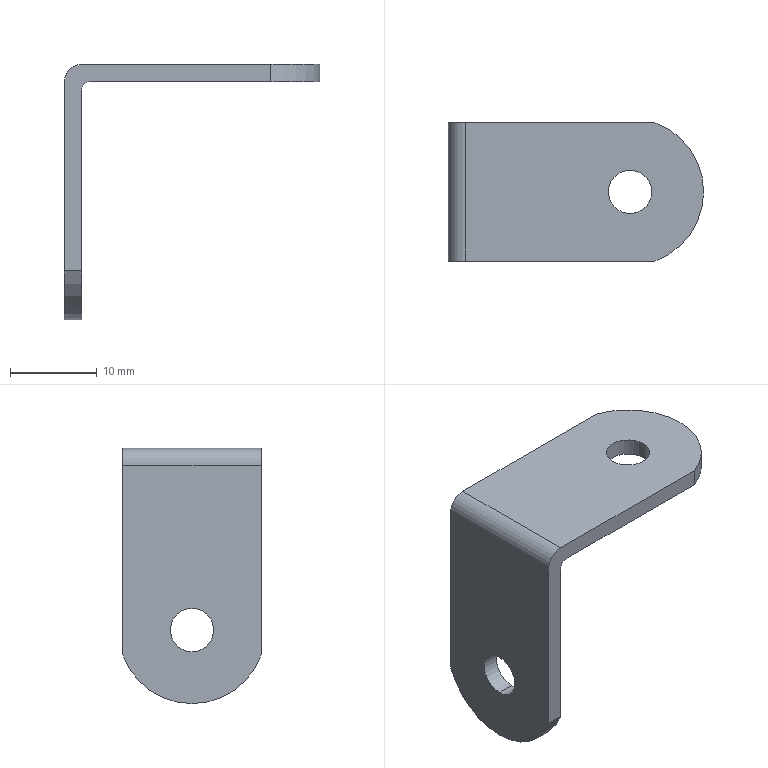Part | SolidWorks | features BaseBody 1 | 1 solid | 15 faces | box 29.5 x 16 x 29.5 mm | volume 1637 mm3 | cylinder 9 | plane 6 | commonest cylinder face diameters 5 x4 17 x3 2 x1 4 x1
STEP:
#1=CARTESIAN_POINT('',(-1.,-8.,-22.872));
#2=VERTEX_POINT('',#1);
#3=CARTESIAN_POINT('',(-1.,0.,-28.5));
#4=VERTEX_POINT('',#3);
#5=CARTESIAN_POINT('',(-1.,0.,-20.));
#6=DIRECTION('',(1.,0.,0.));
#7=DIRECTION('',(0.,0.,-1.));
#8=AXIS2_PLACEMENT_3D('',#5,#6,#7);
#9=CIRCLE('',#8,8.5);
#10=EDGE_CURVE('',#2,#4,#9,.T.);
#11=ORIENTED_EDGE('',*,*,#10,.T.);
#12=CARTESIAN_POINT('',(1.,0.,-28.5));
#13=VERTEX_POINT('',#12);
#14=CARTESIAN_POINT('',(-15.,0.,-28.5));
#15=DIRECTION('',(1.,0.,0.));
#16=VECTOR('',#15,1000.);
#17=LINE('',#14,#16);
#18=EDGE_CURVE('',#4,#13,#17,.T.);
#19=ORIENTED_EDGE('',*,*,#18,.T.);
#20=CARTESIAN_POINT('',(1.,-8.,-22.872));
#21=VERTEX_POINT('',#20);
#22=CARTESIAN_POINT('',(1.,0.,-20.));
#23=DIRECTION('',(-1.,0.,0.));
#24=DIRECTION('',(0.,0.,-1.));
#25=AXIS2_PLACEMENT_3D('',#22,#23,#24);
#26=CIRCLE('',#25,8.5);
#27=EDGE_CURVE('',#13,#21,#26,.T.);
#28=ORIENTED_EDGE('',*,*,#27,.T.);
#29=CARTESIAN_POINT('',(0.,-8.,-22.872));
#30=DIRECTION('',(1.,0.,0.));
#31=VECTOR('',#30,1000.);
#32=LINE('',#29,#31);
#33=EDGE_CURVE('',#2,#21,#32,.T.);
#34=ORIENTED_EDGE('',*,*,#33,.F.);
#35=EDGE_LOOP('',(#11,#19,#28,#34));
#36=FACE_OUTER_BOUND('',#35,.T.);
#37=CARTESIAN_POINT('',(-15.,0.,-20.));
#38=DIRECTION('',(1.,0.,0.));
#39=DIRECTION('',(0.,0.,-1.));
#40=AXIS2_PLACEMENT_3D('',#37,#38,#39);
#41=CYLINDRICAL_SURFACE('',#40,8.5);
#42=ADVANCED_FACE('',(#36),#41,.T.);
#43=CARTESIAN_POINT('',(-1.,0.,-22.5));
#44=VERTEX_POINT('',#43);
#45=CARTESIAN_POINT('',(-1.,0.,-17.5));
#46=VERTEX_POINT('',#45);
#47=CARTESIAN_POINT('',(-1.,0.,-20.));
#48=DIRECTION('',(-1.,0.,0.));
#49=DIRECTION('',(0.,0.,-1.));
#50=AXIS2_PLACEMENT_3D('',#47,#48,#49);
#51=CIRCLE('',#50,2.5);
#52=EDGE_CURVE('',#44,#46,#51,.T.);
#53=ORIENTED_EDGE('',*,*,#52,.T.);
#54=CARTESIAN_POINT('',(1.,0.,-17.5));
#55=VERTEX_POINT('',#54);
#56=CARTESIAN_POINT('',(-15.,0.,-17.5));
#57=DIRECTION('',(1.,0.,0.));
#58=VECTOR('',#57,1000.);
#59=LINE('',#56,#58);
#60=EDGE_CURVE('',#46,#55,#59,.T.);
#61=ORIENTED_EDGE('',*,*,#60,.T.);
#62=CARTESIAN_POINT('',(1.,0.,-22.5));
#63=VERTEX_POINT('',#62);
#64=CARTESIAN_POINT('',(1.,0.,-20.));
#65=DIRECTION('',(-1.,0.,0.));
#66=DIRECTION('',(0.,0.,-1.));
#67=AXIS2_PLACEMENT_3D('',#64,#65,#66);
#68=CIRCLE('',#67,2.5);
#69=EDGE_CURVE('',#63,#55,#68,.T.);
#70=ORIENTED_EDGE('',*,*,#69,.F.);
#71=CARTESIAN_POINT('',(-15.,0.,-22.5));
#72=DIRECTION('',(1.,0.,0.));
#73=VECTOR('',#72,1000.);
#74=LINE('',#71,#73);
#75=EDGE_CURVE('',#44,#63,#74,.T.);
#76=ORIENTED_EDGE('',*,*,#75,.F.);
#77=EDGE_LOOP('',(#53,#61,#70,#76));
#78=FACE_OUTER_BOUND('',#77,.T.);
#79=CARTESIAN_POINT('',(-15.,0.,-20.));
#80=DIRECTION('',(1.,0.,0.));
#81=DIRECTION('',(0.,0.,-1.));
#82=AXIS2_PLACEMENT_3D('',#79,#80,#81);
#83=CYLINDRICAL_SURFACE('',#82,2.5);
#84=ADVANCED_FACE('',(#78),#83,.F.);
#85=CARTESIAN_POINT('',(17.5,0.,1.));
#86=VERTEX_POINT('',#85);
#87=CARTESIAN_POINT('',(22.5,0.,1.));
#88=VERTEX_POINT('',#87);
#89=CARTESIAN_POINT('',(20.,0.,1.));
#90=DIRECTION('',(0.,0.,1.));
#91=DIRECTION('',(-1.,0.,0.));
#92=AXIS2_PLACEMENT_3D('',#89,#90,#91);
#93=CIRCLE('',#92,2.5);
#94=EDGE_CURVE('',#86,#88,#93,.T.);
#95=ORIENTED_EDGE('',*,*,#94,.T.);
#96=CARTESIAN_POINT('',(22.5,0.,-1.));
#97=VERTEX_POINT('',#96);
#98=CARTESIAN_POINT('',(22.5,0.,15.));
#99=DIRECTION('',(0.,0.,-1.));
#100=VECTOR('',#99,1000.);
#101=LINE('',#98,#100);
#102=EDGE_CURVE('',#88,#97,#101,.T.);
#103=ORIENTED_EDGE('',*,*,#102,.T.);
#104=CARTESIAN_POINT('',(17.5,0.,-1.));
#105=VERTEX_POINT('',#104);
#106=CARTESIAN_POINT('',(20.,0.,-1.));
#107=DIRECTION('',(0.,0.,-1.));
#108=DIRECTION('',(-1.,0.,0.));
#109=AXIS2_PLACEMENT_3D('',#106,#107,#108);
#110=CIRCLE('',#109,2.5);
#111=EDGE_CURVE('',#97,#105,#110,.T.);
#112=ORIENTED_EDGE('',*,*,#111,.T.);
#113=CARTESIAN_POINT('',(17.5,0.,15.));
#114=DIRECTION('',(0.,0.,-1.));
#115=VECTOR('',#114,1000.);
#116=LINE('',#113,#115);
#117=EDGE_CURVE('',#86,#105,#116,.T.);
#118=ORIENTED_EDGE('',*,*,#117,.F.);
#119=EDGE_LOOP('',(#95,#103,#112,#118));
#120=FACE_OUTER_BOUND('',#119,.T.);
#121=CARTESIAN_POINT('',(20.,0.,15.));
#122=DIRECTION('',(0.,0.,-1.));
#123=DIRECTION('',(-1.,0.,0.));
#124=AXIS2_PLACEMENT_3D('',#121,#122,#123);
#125=CYLINDRICAL_SURFACE('',#124,2.5);
#126=ADVANCED_FACE('',(#120),#125,.F.);
#127=CARTESIAN_POINT('',(-1.,8.,-1.));
#128=VERTEX_POINT('',#127);
#129=CARTESIAN_POINT('',(-1.,-8.,-1.));
#130=VERTEX_POINT('',#129);
#131=CARTESIAN_POINT('',(-1.,8.,-1.));
#132=DIRECTION('',(0.,-1.,0.));
#133=VECTOR('',#132,1000.);
#134=LINE('',#131,#133);
#135=EDGE_CURVE('',#128,#130,#134,.T.);
#136=ORIENTED_EDGE('',*,*,#135,.F.);
#137=CARTESIAN_POINT('',(-1.,8.,-22.872));
#138=VERTEX_POINT('',#137);
#139=CARTESIAN_POINT('',(-1.,8.,1.));
#140=DIRECTION('',(0.,0.,1.));
#141=VECTOR('',#140,1000.);
#142=LINE('',#139,#141);
#143=EDGE_CURVE('',#138,#128,#142,.T.);
#144=ORIENTED_EDGE('',*,*,#143,.F.);
#145=CARTESIAN_POINT('',(-1.,0.,-20.));
#146=DIRECTION('',(1.,0.,0.));
#147=DIRECTION('',(0.,0.,-1.));
#148=AXIS2_PLACEMENT_3D('',#145,#146,#147);
#149=CIRCLE('',#148,8.5);
#150=EDGE_CURVE('',#4,#138,#149,.T.);
#151=ORIENTED_EDGE('',*,*,#150,.F.);
#152=ORIENTED_EDGE('',*,*,#10,.F.);
#153=CARTESIAN_POINT('',(-1.,-8.,1.));
#154=DIRECTION('',(0.,0.,-1.));
#155=VECTOR('',#154,1000.);
#156=LINE('',#153,#155);
#157=EDGE_CURVE('',#130,#2,#156,.T.);
#158=ORIENTED_EDGE('',*,*,#157,.F.);
#159=EDGE_LOOP('',(#136,#144,#151,#152,#158));
#160=FACE_OUTER_BOUND('',#159,.T.);
#161=ORIENTED_EDGE('',*,*,#52,.F.);
#162=CARTESIAN_POINT('',(-1.,0.,-20.));
#163=DIRECTION('',(-1.,0.,0.));
#164=DIRECTION('',(0.,0.,-1.));
#165=AXIS2_PLACEMENT_3D('',#162,#163,#164);
#166=CIRCLE('',#165,2.5);
#167=EDGE_CURVE('',#46,#44,#166,.T.);
#168=ORIENTED_EDGE('',*,*,#167,.F.);
#169=EDGE_LOOP('',(#161,#168));
#170=FACE_BOUND('',#169,.T.);
#171=CARTESIAN_POINT('',(-1.,8.,1.));
#172=DIRECTION('',(1.,0.,0.));
#173=DIRECTION('',(0.,0.,-1.));
#174=AXIS2_PLACEMENT_3D('',#171,#172,#173);
#175=PLANE('',#174);
#176=ADVANCED_FACE('',(#160,#170),#175,.F.);
#177=CARTESIAN_POINT('',(2.,-8.,-1.));
#178=VERTEX_POINT('',#177);
#179=CARTESIAN_POINT('',(22.872,-8.,-1.));
#180=VERTEX_POINT('',#179);
#181=CARTESIAN_POINT('',(0.,-8.,-1.));
#182=DIRECTION('',(1.,0.,0.));
#183=VECTOR('',#182,1000.);
#184=LINE('',#181,#183);
#185=EDGE_CURVE('',#178,#180,#184,.T.);
#186=ORIENTED_EDGE('',*,*,#185,.T.);
#187=CARTESIAN_POINT('',(22.872,-8.,1.));
#188=VERTEX_POINT('',#187);
#189=CARTESIAN_POINT('',(22.872,-8.,0.));
#190=DIRECTION('',(0.,0.,1.));
#191=VECTOR('',#190,1000.);
#192=LINE('',#189,#191);
#193=EDGE_CURVE('',#180,#188,#192,.T.);
#194=ORIENTED_EDGE('',*,*,#193,.T.);
#195=CARTESIAN_POINT('',(1.,-8.,1.));
#196=VERTEX_POINT('',#195);
#197=CARTESIAN_POINT('',(0.,-8.,1.));
#198=DIRECTION('',(-1.,0.,0.));
#199=VECTOR('',#198,1000.);
#200=LINE('',#197,#199);
#201=EDGE_CURVE('',#188,#196,#200,.T.);
#202=ORIENTED_EDGE('',*,*,#201,.T.);
#203=CARTESIAN_POINT('',(1.,-8.,-1.));
#204=DIRECTION('',(0.,-1.,0.));
#205=DIRECTION('',(0.,0.,-1.));
#206=AXIS2_PLACEMENT_3D('',#203,#204,#205);
#207=CIRCLE('',#206,2.);
#208=EDGE_CURVE('',#196,#130,#207,.T.);
#209=ORIENTED_EDGE('',*,*,#208,.T.);
#210=ORIENTED_EDGE('',*,*,#157,.T.);
#211=ORIENTED_EDGE('',*,*,#33,.T.);
#212=CARTESIAN_POINT('',(1.,-8.,-2.));
#213=VERTEX_POINT('',#212);
#214=CARTESIAN_POINT('',(1.,-8.,0.));
#215=DIRECTION('',(0.,0.,1.));
#216=VECTOR('',#215,1000.);
#217=LINE('',#214,#216);
#218=EDGE_CURVE('',#21,#213,#217,.T.);
#219=ORIENTED_EDGE('',*,*,#218,.T.);
#220=CARTESIAN_POINT('',(2.,-8.,-2.));
#221=DIRECTION('',(0.,1.,0.));
#222=DIRECTION('',(0.,0.,1.));
#223=AXIS2_PLACEMENT_3D('',#220,#221,#222);
#224=CIRCLE('',#223,1.);
#225=EDGE_CURVE('',#213,#178,#224,.T.);
#226=ORIENTED_EDGE('',*,*,#225,.T.);
#227=EDGE_LOOP('',(#186,#194,#202,#209,#210,#211,#219,#226));
#228=FACE_OUTER_BOUND('',#227,.T.);
#229=CARTESIAN_POINT('',(0.,-8.,0.));
#230=DIRECTION('',(0.,-1.,0.));
#231=DIRECTION('',(0.,0.,-1.));
#232=AXIS2_PLACEMENT_3D('',#229,#230,#231);
#233=PLANE('',#232);
#234=ADVANCED_FACE('',(#228),#233,.T.);
#235=ORIENTED_EDGE('',*,*,#208,.F.);
#236=CARTESIAN_POINT('',(1.,8.,1.));
#237=VERTEX_POINT('',#236);
#238=CARTESIAN_POINT('',(1.,8.,1.));
#239=DIRECTION('',(0.,1.,0.));
#240=VECTOR('',#239,1000.);
#241=LINE('',#238,#240);
#242=EDGE_CURVE('',#196,#237,#241,.T.);
#243=ORIENTED_EDGE('',*,*,#242,.T.);
#244=CARTESIAN_POINT('',(1.,8.,-1.));
#245=DIRECTION('',(0.,-1.,0.));
#246=DIRECTION('',(0.,0.,-1.));
#247=AXIS2_PLACEMENT_3D('',#244,#245,#246);
#248=CIRCLE('',#247,2.);
#249=EDGE_CURVE('',#237,#128,#248,.T.);
#250=ORIENTED_EDGE('',*,*,#249,.T.);
#251=ORIENTED_EDGE('',*,*,#135,.T.);
#252=EDGE_LOOP('',(#235,#243,#250,#251));
#253=FACE_OUTER_BOUND('',#252,.T.);
#254=CARTESIAN_POINT('',(1.,8.,-1.));
#255=DIRECTION('',(0.,-1.,0.));
#256=DIRECTION('',(0.,0.,-1.));
#257=AXIS2_PLACEMENT_3D('',#254,#255,#256);
#258=CYLINDRICAL_SURFACE('',#257,2.);
#259=ADVANCED_FACE('',(#253),#258,.T.);
#260=ORIENTED_EDGE('',*,*,#249,.F.);
#261=CARTESIAN_POINT('',(22.872,8.,1.));
#262=VERTEX_POINT('',#261);
#263=CARTESIAN_POINT('',(0.,8.,1.));
#264=DIRECTION('',(-1.,0.,0.));
#265=VECTOR('',#264,1000.);
#266=LINE('',#263,#265);
#267=EDGE_CURVE('',#262,#237,#266,.T.);
#268=ORIENTED_EDGE('',*,*,#267,.F.);
#269=CARTESIAN_POINT('',(22.872,8.,-1.));
#270=VERTEX_POINT('',#269);
#271=CARTESIAN_POINT('',(22.872,8.,0.));
#272=DIRECTION('',(0.,0.,1.));
#273=VECTOR('',#272,1000.);
#274=LINE('',#271,#273);
#275=EDGE_CURVE('',#270,#262,#274,.T.);
#276=ORIENTED_EDGE('',*,*,#275,.F.);
#277=CARTESIAN_POINT('',(2.,8.,-1.));
#278=VERTEX_POINT('',#277);
#279=CARTESIAN_POINT('',(0.,8.,-1.));
#280=DIRECTION('',(1.,0.,0.));
#281=VECTOR('',#280,1000.);
#282=LINE('',#279,#281);
#283=EDGE_CURVE('',#278,#270,#282,.T.);
#284=ORIENTED_EDGE('',*,*,#283,.F.);
#285=CARTESIAN_POINT('',(1.,8.,-2.));
#286=VERTEX_POINT('',#285);
#287=CARTESIAN_POINT('',(2.,8.,-2.));
#288=DIRECTION('',(0.,-1.,0.));
#289=DIRECTION('',(0.,0.,1.));
#290=AXIS2_PLACEMENT_3D('',#287,#288,#289);
#291=CIRCLE('',#290,1.);
#292=EDGE_CURVE('',#278,#286,#291,.T.);
#293=ORIENTED_EDGE('',*,*,#292,.T.);
#294=CARTESIAN_POINT('',(1.,8.,-22.872));
#295=VERTEX_POINT('',#294);
#296=CARTESIAN_POINT('',(1.,8.,0.));
#297=DIRECTION('',(0.,0.,1.));
#298=VECTOR('',#297,1000.);
#299=LINE('',#296,#298);
#300=EDGE_CURVE('',#295,#286,#299,.T.);
#301=ORIENTED_EDGE('',*,*,#300,.F.);
#302=CARTESIAN_POINT('',(0.,8.,-22.872));
#303=DIRECTION('',(1.,0.,0.));
#304=VECTOR('',#303,1000.);
#305=LINE('',#302,#304);
#306=EDGE_CURVE('',#138,#295,#305,.T.);
#307=ORIENTED_EDGE('',*,*,#306,.F.);
#308=ORIENTED_EDGE('',*,*,#143,.T.);
#309=EDGE_LOOP('',(#260,#268,#276,#284,#293,#301,#307,#308));
#310=FACE_OUTER_BOUND('',#309,.T.);
#311=CARTESIAN_POINT('',(0.,8.,0.));
#312=DIRECTION('',(0.,-1.,0.));
#313=DIRECTION('',(0.,0.,-1.));
#314=AXIS2_PLACEMENT_3D('',#311,#312,#313);
#315=PLANE('',#314);
#316=ADVANCED_FACE('',(#310),#315,.F.);
#317=ORIENTED_EDGE('',*,*,#18,.F.);
#318=ORIENTED_EDGE('',*,*,#150,.T.);
#319=ORIENTED_EDGE('',*,*,#306,.T.);
#320=CARTESIAN_POINT('',(1.,0.,-20.));
#321=DIRECTION('',(-1.,0.,0.));
#322=DIRECTION('',(0.,0.,-1.));
#323=AXIS2_PLACEMENT_3D('',#320,#321,#322);
#324=CIRCLE('',#323,8.5);
#325=EDGE_CURVE('',#295,#13,#324,.T.);
#326=ORIENTED_EDGE('',*,*,#325,.T.);
#327=EDGE_LOOP('',(#317,#318,#319,#326));
#328=FACE_OUTER_BOUND('',#327,.T.);
#329=CARTESIAN_POINT('',(-15.,0.,-20.));
#330=DIRECTION('',(1.,0.,0.));
#331=DIRECTION('',(0.,0.,-1.));
#332=AXIS2_PLACEMENT_3D('',#329,#330,#331);
#333=CYLINDRICAL_SURFACE('',#332,8.5);
#334=ADVANCED_FACE('',(#328),#333,.T.);
#335=ORIENTED_EDGE('',*,*,#60,.F.);
#336=ORIENTED_EDGE('',*,*,#167,.T.);
#337=ORIENTED_EDGE('',*,*,#75,.T.);
#338=CARTESIAN_POINT('',(1.,0.,-20.));
#339=DIRECTION('',(-1.,0.,0.));
#340=DIRECTION('',(0.,0.,-1.));
#341=AXIS2_PLACEMENT_3D('',#338,#339,#340);
#342=CIRCLE('',#341,2.5);
#343=EDGE_CURVE('',#55,#63,#342,.T.);
#344=ORIENTED_EDGE('',*,*,#343,.F.);
#345=EDGE_LOOP('',(#335,#336,#337,#344));
#346=FACE_OUTER_BOUND('',#345,.T.);
#347=CARTESIAN_POINT('',(-15.,0.,-20.));
#348=DIRECTION('',(1.,0.,0.));
#349=DIRECTION('',(0.,0.,-1.));
#350=AXIS2_PLACEMENT_3D('',#347,#348,#349);
#351=CYLINDRICAL_SURFACE('',#350,2.5);
#352=ADVANCED_FACE('',(#346),#351,.F.);
#353=ORIENTED_EDGE('',*,*,#275,.T.);
#354=CARTESIAN_POINT('',(20.,0.,1.));
#355=DIRECTION('',(0.,0.,-1.));
#356=DIRECTION('',(-1.,0.,0.));
#357=AXIS2_PLACEMENT_3D('',#354,#355,#356);
#358=CIRCLE('',#357,8.5);
#359=EDGE_CURVE('',#262,#188,#358,.T.);
#360=ORIENTED_EDGE('',*,*,#359,.T.);
#361=ORIENTED_EDGE('',*,*,#193,.F.);
#362=CARTESIAN_POINT('',(20.,0.,-1.));
#363=DIRECTION('',(0.,0.,1.));
#364=DIRECTION('',(-1.,0.,0.));
#365=AXIS2_PLACEMENT_3D('',#362,#363,#364);
#366=CIRCLE('',#365,8.5);
#367=EDGE_CURVE('',#180,#270,#366,.T.);
#368=ORIENTED_EDGE('',*,*,#367,.T.);
#369=EDGE_LOOP('',(#353,#360,#361,#368));
#370=FACE_OUTER_BOUND('',#369,.T.);
#371=CARTESIAN_POINT('',(20.,0.,15.));
#372=DIRECTION('',(0.,0.,-1.));
#373=DIRECTION('',(-1.,0.,0.));
#374=AXIS2_PLACEMENT_3D('',#371,#372,#373);
#375=CYLINDRICAL_SURFACE('',#374,8.5);
#376=ADVANCED_FACE('',(#370),#375,.T.);
#377=CARTESIAN_POINT('',(2.,8.,-1.));
#378=DIRECTION('',(0.,-1.,0.));
#379=VECTOR('',#378,1000.);
#380=LINE('',#377,#379);
#381=EDGE_CURVE('',#278,#178,#380,.T.);
#382=ORIENTED_EDGE('',*,*,#381,.F.);
#383=ORIENTED_EDGE('',*,*,#283,.T.);
#384=ORIENTED_EDGE('',*,*,#367,.F.);
#385=ORIENTED_EDGE('',*,*,#185,.F.);
#386=EDGE_LOOP('',(#382,#383,#384,#385));
#387=FACE_OUTER_BOUND('',#386,.T.);
#388=CARTESIAN_POINT('',(20.,0.,-1.));
#389=DIRECTION('',(0.,0.,-1.));
#390=DIRECTION('',(-1.,0.,0.));
#391=AXIS2_PLACEMENT_3D('',#388,#389,#390);
#392=CIRCLE('',#391,2.5);
#393=EDGE_CURVE('',#105,#97,#392,.T.);
#394=ORIENTED_EDGE('',*,*,#393,.F.);
#395=ORIENTED_EDGE('',*,*,#111,.F.);
#396=EDGE_LOOP('',(#394,#395));
#397=FACE_BOUND('',#396,.T.);
#398=CARTESIAN_POINT('',(1.,8.,-1.));
#399=DIRECTION('',(0.,0.,1.));
#400=DIRECTION('',(1.,0.,0.));
#401=AXIS2_PLACEMENT_3D('',#398,#399,#400);
#402=PLANE('',#401);
#403=ADVANCED_FACE('',(#387,#397),#402,.F.);
#404=CARTESIAN_POINT('',(1.,8.,-2.));
#405=DIRECTION('',(0.,1.,0.));
#406=VECTOR('',#405,1000.);
#407=LINE('',#404,#406);
#408=EDGE_CURVE('',#213,#286,#407,.T.);
#409=ORIENTED_EDGE('',*,*,#408,.F.);
#410=ORIENTED_EDGE('',*,*,#218,.F.);
#411=ORIENTED_EDGE('',*,*,#27,.F.);
#412=ORIENTED_EDGE('',*,*,#325,.F.);
#413=ORIENTED_EDGE('',*,*,#300,.T.);
#414=EDGE_LOOP('',(#409,#410,#411,#412,#413));
#415=FACE_OUTER_BOUND('',#414,.T.);
#416=ORIENTED_EDGE('',*,*,#69,.T.);
#417=ORIENTED_EDGE('',*,*,#343,.T.);
#418=EDGE_LOOP('',(#416,#417));
#419=FACE_BOUND('',#418,.T.);
#420=CARTESIAN_POINT('',(1.,8.,-1.));
#421=DIRECTION('',(-1.,0.,0.));
#422=DIRECTION('',(0.,0.,1.));
#423=AXIS2_PLACEMENT_3D('',#420,#421,#422);
#424=PLANE('',#423);
#425=ADVANCED_FACE('',(#415,#419),#424,.F.);
#426=ORIENTED_EDGE('',*,*,#242,.F.);
#427=ORIENTED_EDGE('',*,*,#201,.F.);
#428=ORIENTED_EDGE('',*,*,#359,.F.);
#429=ORIENTED_EDGE('',*,*,#267,.T.);
#430=EDGE_LOOP('',(#426,#427,#428,#429));
#431=FACE_OUTER_BOUND('',#430,.T.);
#432=ORIENTED_EDGE('',*,*,#94,.F.);
#433=CARTESIAN_POINT('',(20.,0.,1.));
#434=DIRECTION('',(0.,0.,1.));
#435=DIRECTION('',(-1.,0.,0.));
#436=AXIS2_PLACEMENT_3D('',#433,#434,#435);
#437=CIRCLE('',#436,2.5);
#438=EDGE_CURVE('',#88,#86,#437,.T.);
#439=ORIENTED_EDGE('',*,*,#438,.F.);
#440=EDGE_LOOP('',(#432,#439));
#441=FACE_BOUND('',#440,.T.);
#442=CARTESIAN_POINT('',(-1.,8.,1.));
#443=DIRECTION('',(0.,0.,-1.));
#444=DIRECTION('',(-1.,0.,0.));
#445=AXIS2_PLACEMENT_3D('',#442,#443,#444);
#446=PLANE('',#445);
#447=ADVANCED_FACE('',(#431,#441),#446,.F.);
#448=ORIENTED_EDGE('',*,*,#381,.T.);
#449=ORIENTED_EDGE('',*,*,#225,.F.);
#450=ORIENTED_EDGE('',*,*,#408,.T.);
#451=ORIENTED_EDGE('',*,*,#292,.F.);
#452=EDGE_LOOP('',(#448,#449,#450,#451));
#453=FACE_OUTER_BOUND('',#452,.T.);
#454=CARTESIAN_POINT('',(2.,8.,-2.));
#455=DIRECTION('',(0.,1.,0.));
#456=DIRECTION('',(0.,0.,1.));
#457=AXIS2_PLACEMENT_3D('',#454,#455,#456);
#458=CYLINDRICAL_SURFACE('',#457,1.);
#459=ADVANCED_FACE('',(#453),#458,.F.);
#460=ORIENTED_EDGE('',*,*,#102,.F.);
#461=ORIENTED_EDGE('',*,*,#438,.T.);
#462=ORIENTED_EDGE('',*,*,#117,.T.);
#463=ORIENTED_EDGE('',*,*,#393,.T.);
#464=EDGE_LOOP('',(#460,#461,#462,#463));
#465=FACE_OUTER_BOUND('',#464,.T.);
#466=CARTESIAN_POINT('',(20.,0.,15.));
#467=DIRECTION('',(0.,0.,-1.));
#468=DIRECTION('',(-1.,0.,0.));
#469=AXIS2_PLACEMENT_3D('',#466,#467,#468);
#470=CYLINDRICAL_SURFACE('',#469,2.5);
#471=ADVANCED_FACE('',(#465),#470,.F.);
#472=CLOSED_SHELL('',(#42,#84,#126,#176,#234,#259,#316,#334,#352,#376,#403,#425,#447,#459,#471));
#473=MANIFOLD_SOLID_BREP('',#472);
#474=CARTESIAN_POINT('',(0.,0.,0.));
#475=DIRECTION('',(0.,0.,1.));
#476=DIRECTION('',(1.,0.,0.));
#477=AXIS2_PLACEMENT_3D('',#474,#475,#476);
#478=(LENGTH_UNIT()NAMED_UNIT(*)SI_UNIT(.MILLI.,.METRE.));
#479=UNCERTAINTY_MEASURE_WITH_UNIT(LENGTH_MEASURE(0.00001),#478,'','');
#480=(NAMED_UNIT(*)PLANE_ANGLE_UNIT()SI_UNIT($,.RADIAN.));
#481=(NAMED_UNIT(*)SI_UNIT($,.STERADIAN.)SOLID_ANGLE_UNIT());
#482=(GEOMETRIC_REPRESENTATION_CONTEXT(3)GLOBAL_UNCERTAINTY_ASSIGNED_CONTEXT((#479))GLOBAL_UNIT_ASSIGNED_CONTEXT((#478,#480,#481))REPRESENTATION_CONTEXT('',''));
#483=ADVANCED_BREP_SHAPE_REPRESENTATION('',(#473,#477),#482);